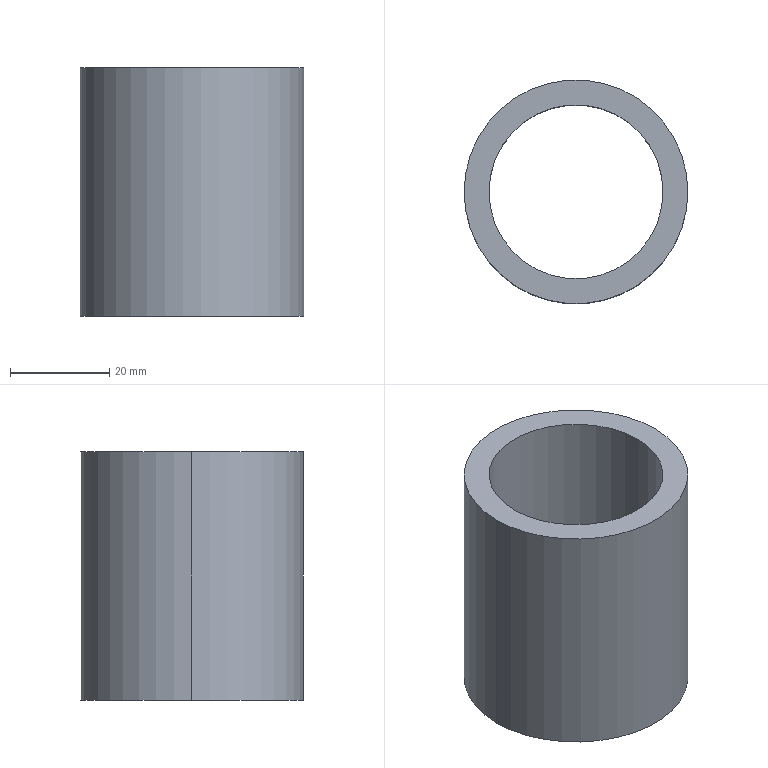Part | SolidWorks | features ICE 2, Extrusion 1 | 1 solid | 6 faces | box 45 x 45 x 50 mm | volume 31416 mm3 | cylinder 4 | plane 2 | commonest cylinder face diameters 35 x2 45 x2
STEP:
#1=CARTESIAN_POINT('',(-17.5,0.,0.));
#2=VERTEX_POINT('',#1);
#3=CARTESIAN_POINT('',(17.5,0.,0.));
#4=VERTEX_POINT('',#3);
#5=CARTESIAN_POINT('',(0.,0.,0.));
#6=DIRECTION('',(0.,0.,1.));
#7=DIRECTION('',(1.,0.,0.));
#8=AXIS2_PLACEMENT_3D('',#5,#6,#7);
#9=CIRCLE('',#8,17.5);
#10=EDGE_CURVE('',#2,#4,#9,.T.);
#11=ORIENTED_EDGE('',*,*,#10,.F.);
#12=CARTESIAN_POINT('',(-17.5,0.,50.));
#13=VERTEX_POINT('',#12);
#14=CARTESIAN_POINT('',(-17.5,0.,0.));
#15=DIRECTION('',(0.,0.,1.));
#16=VECTOR('',#15,1000.);
#17=LINE('',#14,#16);
#18=EDGE_CURVE('',#2,#13,#17,.T.);
#19=ORIENTED_EDGE('',*,*,#18,.T.);
#20=CARTESIAN_POINT('',(17.5,0.,50.));
#21=VERTEX_POINT('',#20);
#22=CARTESIAN_POINT('',(0.,0.,50.));
#23=DIRECTION('',(0.,0.,1.));
#24=DIRECTION('',(1.,0.,0.));
#25=AXIS2_PLACEMENT_3D('',#22,#23,#24);
#26=CIRCLE('',#25,17.5);
#27=EDGE_CURVE('',#13,#21,#26,.T.);
#28=ORIENTED_EDGE('',*,*,#27,.T.);
#29=CARTESIAN_POINT('',(17.5,0.,0.));
#30=DIRECTION('',(0.,0.,1.));
#31=VECTOR('',#30,1000.);
#32=LINE('',#29,#31);
#33=EDGE_CURVE('',#4,#21,#32,.T.);
#34=ORIENTED_EDGE('',*,*,#33,.F.);
#35=EDGE_LOOP('',(#11,#19,#28,#34));
#36=FACE_OUTER_BOUND('',#35,.T.);
#37=CARTESIAN_POINT('',(0.,0.,0.));
#38=DIRECTION('',(0.,0.,1.));
#39=DIRECTION('',(1.,0.,0.));
#40=AXIS2_PLACEMENT_3D('',#37,#38,#39);
#41=CYLINDRICAL_SURFACE('',#40,17.5);
#42=ADVANCED_FACE('',(#36),#41,.F.);
#43=CARTESIAN_POINT('',(22.5,0.,0.));
#44=VERTEX_POINT('',#43);
#45=CARTESIAN_POINT('',(-22.5,0.,0.));
#46=VERTEX_POINT('',#45);
#47=CARTESIAN_POINT('',(0.,0.,0.));
#48=DIRECTION('',(0.,0.,1.));
#49=DIRECTION('',(1.,0.,0.));
#50=AXIS2_PLACEMENT_3D('',#47,#48,#49);
#51=CIRCLE('',#50,22.5);
#52=EDGE_CURVE('',#44,#46,#51,.T.);
#53=ORIENTED_EDGE('',*,*,#52,.T.);
#54=CARTESIAN_POINT('',(-22.5,0.,50.));
#55=VERTEX_POINT('',#54);
#56=CARTESIAN_POINT('',(-22.5,0.,0.));
#57=DIRECTION('',(0.,0.,1.));
#58=VECTOR('',#57,1000.);
#59=LINE('',#56,#58);
#60=EDGE_CURVE('',#46,#55,#59,.T.);
#61=ORIENTED_EDGE('',*,*,#60,.T.);
#62=CARTESIAN_POINT('',(22.5,0.,50.));
#63=VERTEX_POINT('',#62);
#64=CARTESIAN_POINT('',(0.,0.,50.));
#65=DIRECTION('',(0.,0.,1.));
#66=DIRECTION('',(1.,0.,0.));
#67=AXIS2_PLACEMENT_3D('',#64,#65,#66);
#68=CIRCLE('',#67,22.5);
#69=EDGE_CURVE('',#63,#55,#68,.T.);
#70=ORIENTED_EDGE('',*,*,#69,.F.);
#71=CARTESIAN_POINT('',(22.5,0.,0.));
#72=DIRECTION('',(0.,0.,1.));
#73=VECTOR('',#72,1000.);
#74=LINE('',#71,#73);
#75=EDGE_CURVE('',#44,#63,#74,.T.);
#76=ORIENTED_EDGE('',*,*,#75,.F.);
#77=EDGE_LOOP('',(#53,#61,#70,#76));
#78=FACE_OUTER_BOUND('',#77,.T.);
#79=CARTESIAN_POINT('',(0.,0.,0.));
#80=DIRECTION('',(0.,0.,1.));
#81=DIRECTION('',(1.,0.,0.));
#82=AXIS2_PLACEMENT_3D('',#79,#80,#81);
#83=CYLINDRICAL_SURFACE('',#82,22.5);
#84=ADVANCED_FACE('',(#78),#83,.T.);
#85=CARTESIAN_POINT('',(0.,0.,50.));
#86=DIRECTION('',(0.,0.,1.));
#87=DIRECTION('',(1.,0.,0.));
#88=AXIS2_PLACEMENT_3D('',#85,#86,#87);
#89=CIRCLE('',#88,17.5);
#90=EDGE_CURVE('',#21,#13,#89,.T.);
#91=ORIENTED_EDGE('',*,*,#90,.F.);
#92=ORIENTED_EDGE('',*,*,#27,.F.);
#93=EDGE_LOOP('',(#91,#92));
#94=FACE_BOUND('',#93,.T.);
#95=ORIENTED_EDGE('',*,*,#69,.T.);
#96=CARTESIAN_POINT('',(0.,0.,50.));
#97=DIRECTION('',(0.,0.,1.));
#98=DIRECTION('',(1.,0.,0.));
#99=AXIS2_PLACEMENT_3D('',#96,#97,#98);
#100=CIRCLE('',#99,22.5);
#101=EDGE_CURVE('',#55,#63,#100,.T.);
#102=ORIENTED_EDGE('',*,*,#101,.T.);
#103=EDGE_LOOP('',(#95,#102));
#104=FACE_OUTER_BOUND('',#103,.T.);
#105=CARTESIAN_POINT('',(0.,0.,50.));
#106=DIRECTION('',(0.,0.,1.));
#107=DIRECTION('',(1.,0.,0.));
#108=AXIS2_PLACEMENT_3D('',#105,#106,#107);
#109=PLANE('',#108);
#110=ADVANCED_FACE('',(#94,#104),#109,.T.);
#111=CARTESIAN_POINT('',(0.,0.,0.));
#112=DIRECTION('',(0.,0.,1.));
#113=DIRECTION('',(1.,0.,0.));
#114=AXIS2_PLACEMENT_3D('',#111,#112,#113);
#115=CIRCLE('',#114,17.5);
#116=EDGE_CURVE('',#4,#2,#115,.T.);
#117=ORIENTED_EDGE('',*,*,#116,.T.);
#118=ORIENTED_EDGE('',*,*,#10,.T.);
#119=EDGE_LOOP('',(#117,#118));
#120=FACE_BOUND('',#119,.T.);
#121=ORIENTED_EDGE('',*,*,#52,.F.);
#122=CARTESIAN_POINT('',(0.,0.,0.));
#123=DIRECTION('',(0.,0.,1.));
#124=DIRECTION('',(1.,0.,0.));
#125=AXIS2_PLACEMENT_3D('',#122,#123,#124);
#126=CIRCLE('',#125,22.5);
#127=EDGE_CURVE('',#46,#44,#126,.T.);
#128=ORIENTED_EDGE('',*,*,#127,.F.);
#129=EDGE_LOOP('',(#121,#128));
#130=FACE_OUTER_BOUND('',#129,.T.);
#131=CARTESIAN_POINT('',(0.,0.,0.));
#132=DIRECTION('',(0.,0.,1.));
#133=DIRECTION('',(1.,0.,0.));
#134=AXIS2_PLACEMENT_3D('',#131,#132,#133);
#135=PLANE('',#134);
#136=ADVANCED_FACE('',(#120,#130),#135,.F.);
#137=ORIENTED_EDGE('',*,*,#60,.F.);
#138=ORIENTED_EDGE('',*,*,#127,.T.);
#139=ORIENTED_EDGE('',*,*,#75,.T.);
#140=ORIENTED_EDGE('',*,*,#101,.F.);
#141=EDGE_LOOP('',(#137,#138,#139,#140));
#142=FACE_OUTER_BOUND('',#141,.T.);
#143=CARTESIAN_POINT('',(0.,0.,0.));
#144=DIRECTION('',(0.,0.,1.));
#145=DIRECTION('',(1.,0.,0.));
#146=AXIS2_PLACEMENT_3D('',#143,#144,#145);
#147=CYLINDRICAL_SURFACE('',#146,22.5);
#148=ADVANCED_FACE('',(#142),#147,.T.);
#149=ORIENTED_EDGE('',*,*,#18,.F.);
#150=ORIENTED_EDGE('',*,*,#116,.F.);
#151=ORIENTED_EDGE('',*,*,#33,.T.);
#152=ORIENTED_EDGE('',*,*,#90,.T.);
#153=EDGE_LOOP('',(#149,#150,#151,#152));
#154=FACE_OUTER_BOUND('',#153,.T.);
#155=CARTESIAN_POINT('',(0.,0.,0.));
#156=DIRECTION('',(0.,0.,1.));
#157=DIRECTION('',(1.,0.,0.));
#158=AXIS2_PLACEMENT_3D('',#155,#156,#157);
#159=CYLINDRICAL_SURFACE('',#158,17.5);
#160=ADVANCED_FACE('',(#154),#159,.F.);
#161=CLOSED_SHELL('',(#42,#84,#110,#136,#148,#160));
#162=MANIFOLD_SOLID_BREP('',#161);
#163=CARTESIAN_POINT('',(0.,0.,0.));
#164=DIRECTION('',(0.,0.,1.));
#165=DIRECTION('',(1.,0.,0.));
#166=AXIS2_PLACEMENT_3D('',#163,#164,#165);
#167=(LENGTH_UNIT()NAMED_UNIT(*)SI_UNIT(.MILLI.,.METRE.));
#168=UNCERTAINTY_MEASURE_WITH_UNIT(LENGTH_MEASURE(0.00001),#167,'','');
#169=(NAMED_UNIT(*)PLANE_ANGLE_UNIT()SI_UNIT($,.RADIAN.));
#170=(NAMED_UNIT(*)SI_UNIT($,.STERADIAN.)SOLID_ANGLE_UNIT());
#171=(GEOMETRIC_REPRESENTATION_CONTEXT(3)GLOBAL_UNCERTAINTY_ASSIGNED_CONTEXT((#168))GLOBAL_UNIT_ASSIGNED_CONTEXT((#167,#169,#170))REPRESENTATION_CONTEXT('',''));
#172=ADVANCED_BREP_SHAPE_REPRESENTATION('',(#162,#166),#171);